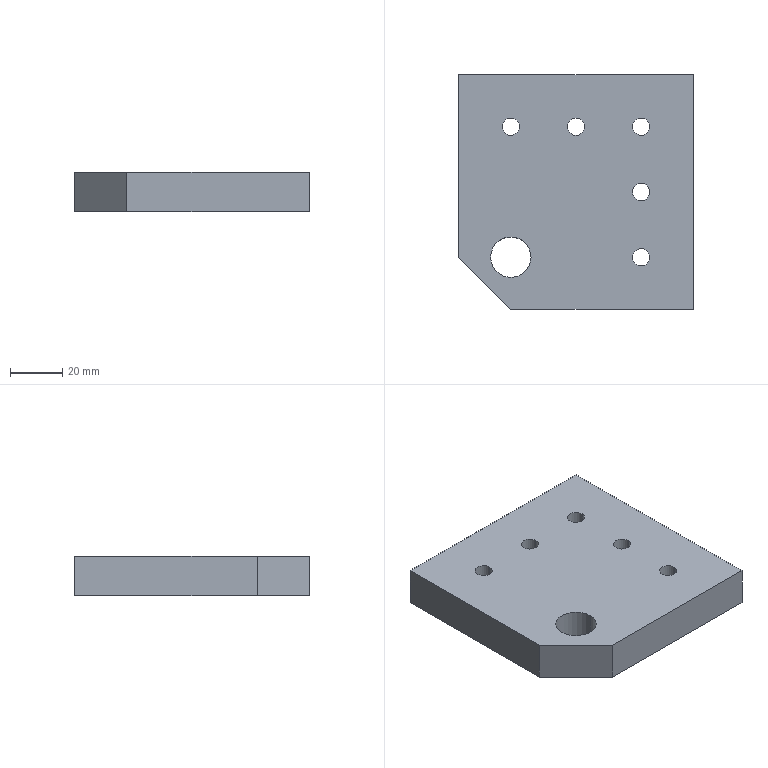Part | SolidWorks | features BaseBody 1 | 1 solid | 34 faces | box 90 x 90 x 15 mm | volume 110422 mm3 | cylinder 22 | plane 12 | commonest cylinder face diameters 6.6 x10 12 x10 15.5 x2
STEP:
#1=CARTESIAN_POINT('',(31.,25.,6.8));
#2=VERTEX_POINT('',#1);
#3=CARTESIAN_POINT('',(19.,25.,6.8));
#4=VERTEX_POINT('',#3);
#5=CARTESIAN_POINT('',(25.,25.,6.8));
#6=DIRECTION('',(0.,0.,-1.));
#7=DIRECTION('',(-1.,0.,0.));
#8=AXIS2_PLACEMENT_3D('',#5,#6,#7);
#9=CIRCLE('',#8,6.);
#10=EDGE_CURVE('',#2,#4,#9,.T.);
#11=ORIENTED_EDGE('',*,*,#10,.F.);
#12=CARTESIAN_POINT('',(31.,25.,0.));
#13=VERTEX_POINT('',#12);
#14=CARTESIAN_POINT('',(31.,25.,0.));
#15=DIRECTION('',(0.,0.,-1.));
#16=VECTOR('',#15,1000.);
#17=LINE('',#14,#16);
#18=EDGE_CURVE('',#2,#13,#17,.T.);
#19=ORIENTED_EDGE('',*,*,#18,.T.);
#20=CARTESIAN_POINT('',(19.,25.,0.));
#21=VERTEX_POINT('',#20);
#22=CARTESIAN_POINT('',(25.,25.,0.));
#23=DIRECTION('',(0.,0.,-1.));
#24=DIRECTION('',(-1.,0.,0.));
#25=AXIS2_PLACEMENT_3D('',#22,#23,#24);
#26=CIRCLE('',#25,6.);
#27=EDGE_CURVE('',#13,#21,#26,.T.);
#28=ORIENTED_EDGE('',*,*,#27,.T.);
#29=CARTESIAN_POINT('',(19.,25.,0.));
#30=DIRECTION('',(0.,0.,-1.));
#31=VECTOR('',#30,1000.);
#32=LINE('',#29,#31);
#33=EDGE_CURVE('',#4,#21,#32,.T.);
#34=ORIENTED_EDGE('',*,*,#33,.F.);
#35=EDGE_LOOP('',(#11,#19,#28,#34));
#36=FACE_OUTER_BOUND('',#35,.T.);
#37=CARTESIAN_POINT('',(25.,25.,0.));
#38=DIRECTION('',(0.,0.,-1.));
#39=DIRECTION('',(-1.,0.,0.));
#40=AXIS2_PLACEMENT_3D('',#37,#38,#39);
#41=CYLINDRICAL_SURFACE('',#40,6.);
#42=ADVANCED_FACE('',(#36),#41,.F.);
#43=CARTESIAN_POINT('',(28.3,25.,15.));
#44=VERTEX_POINT('',#43);
#45=CARTESIAN_POINT('',(21.7,25.,15.));
#46=VERTEX_POINT('',#45);
#47=CARTESIAN_POINT('',(25.,25.,15.));
#48=DIRECTION('',(0.,0.,-1.));
#49=DIRECTION('',(-1.,0.,0.));
#50=AXIS2_PLACEMENT_3D('',#47,#48,#49);
#51=CIRCLE('',#50,3.3);
#52=EDGE_CURVE('',#44,#46,#51,.T.);
#53=ORIENTED_EDGE('',*,*,#52,.F.);
#54=CARTESIAN_POINT('',(28.3,25.,6.8));
#55=VERTEX_POINT('',#54);
#56=CARTESIAN_POINT('',(28.3,25.,0.));
#57=DIRECTION('',(0.,0.,-1.));
#58=VECTOR('',#57,1000.);
#59=LINE('',#56,#58);
#60=EDGE_CURVE('',#44,#55,#59,.T.);
#61=ORIENTED_EDGE('',*,*,#60,.T.);
#62=CARTESIAN_POINT('',(21.7,25.,6.8));
#63=VERTEX_POINT('',#62);
#64=CARTESIAN_POINT('',(25.,25.,6.8));
#65=DIRECTION('',(0.,0.,-1.));
#66=DIRECTION('',(-1.,0.,0.));
#67=AXIS2_PLACEMENT_3D('',#64,#65,#66);
#68=CIRCLE('',#67,3.3);
#69=EDGE_CURVE('',#55,#63,#68,.T.);
#70=ORIENTED_EDGE('',*,*,#69,.T.);
#71=CARTESIAN_POINT('',(21.7,25.,0.));
#72=DIRECTION('',(0.,0.,-1.));
#73=VECTOR('',#72,1000.);
#74=LINE('',#71,#73);
#75=EDGE_CURVE('',#46,#63,#74,.T.);
#76=ORIENTED_EDGE('',*,*,#75,.F.);
#77=EDGE_LOOP('',(#53,#61,#70,#76));
#78=FACE_OUTER_BOUND('',#77,.T.);
#79=CARTESIAN_POINT('',(25.,25.,0.));
#80=DIRECTION('',(0.,0.,-1.));
#81=DIRECTION('',(-1.,0.,0.));
#82=AXIS2_PLACEMENT_3D('',#79,#80,#81);
#83=CYLINDRICAL_SURFACE('',#82,3.3);
#84=ADVANCED_FACE('',(#78),#83,.F.);
#85=CARTESIAN_POINT('',(6.,25.,6.8));
#86=VERTEX_POINT('',#85);
#87=CARTESIAN_POINT('',(-6.,25.,6.8));
#88=VERTEX_POINT('',#87);
#89=CARTESIAN_POINT('',(0.,25.,6.8));
#90=DIRECTION('',(0.,0.,-1.));
#91=DIRECTION('',(-1.,0.,0.));
#92=AXIS2_PLACEMENT_3D('',#89,#90,#91);
#93=CIRCLE('',#92,6.);
#94=EDGE_CURVE('',#86,#88,#93,.T.);
#95=ORIENTED_EDGE('',*,*,#94,.F.);
#96=CARTESIAN_POINT('',(6.,25.,0.));
#97=VERTEX_POINT('',#96);
#98=CARTESIAN_POINT('',(6.,25.,0.));
#99=DIRECTION('',(0.,0.,-1.));
#100=VECTOR('',#99,1000.);
#101=LINE('',#98,#100);
#102=EDGE_CURVE('',#86,#97,#101,.T.);
#103=ORIENTED_EDGE('',*,*,#102,.T.);
#104=CARTESIAN_POINT('',(-6.,25.,0.));
#105=VERTEX_POINT('',#104);
#106=CARTESIAN_POINT('',(0.,25.,0.));
#107=DIRECTION('',(0.,0.,-1.));
#108=DIRECTION('',(-1.,0.,0.));
#109=AXIS2_PLACEMENT_3D('',#106,#107,#108);
#110=CIRCLE('',#109,6.);
#111=EDGE_CURVE('',#97,#105,#110,.T.);
#112=ORIENTED_EDGE('',*,*,#111,.T.);
#113=CARTESIAN_POINT('',(-6.,25.,0.));
#114=DIRECTION('',(0.,0.,-1.));
#115=VECTOR('',#114,1000.);
#116=LINE('',#113,#115);
#117=EDGE_CURVE('',#88,#105,#116,.T.);
#118=ORIENTED_EDGE('',*,*,#117,.F.);
#119=EDGE_LOOP('',(#95,#103,#112,#118));
#120=FACE_OUTER_BOUND('',#119,.T.);
#121=CARTESIAN_POINT('',(0.,25.,0.));
#122=DIRECTION('',(0.,0.,-1.));
#123=DIRECTION('',(-1.,0.,0.));
#124=AXIS2_PLACEMENT_3D('',#121,#122,#123);
#125=CYLINDRICAL_SURFACE('',#124,6.);
#126=ADVANCED_FACE('',(#120),#125,.F.);
#127=CARTESIAN_POINT('',(3.3,25.,15.));
#128=VERTEX_POINT('',#127);
#129=CARTESIAN_POINT('',(-3.3,25.,15.));
#130=VERTEX_POINT('',#129);
#131=CARTESIAN_POINT('',(0.,25.,15.));
#132=DIRECTION('',(0.,0.,-1.));
#133=DIRECTION('',(-1.,0.,0.));
#134=AXIS2_PLACEMENT_3D('',#131,#132,#133);
#135=CIRCLE('',#134,3.3);
#136=EDGE_CURVE('',#128,#130,#135,.T.);
#137=ORIENTED_EDGE('',*,*,#136,.F.);
#138=CARTESIAN_POINT('',(3.3,25.,6.8));
#139=VERTEX_POINT('',#138);
#140=CARTESIAN_POINT('',(3.3,25.,0.));
#141=DIRECTION('',(0.,0.,-1.));
#142=VECTOR('',#141,1000.);
#143=LINE('',#140,#142);
#144=EDGE_CURVE('',#128,#139,#143,.T.);
#145=ORIENTED_EDGE('',*,*,#144,.T.);
#146=CARTESIAN_POINT('',(-3.3,25.,6.8));
#147=VERTEX_POINT('',#146);
#148=CARTESIAN_POINT('',(0.,25.,6.8));
#149=DIRECTION('',(0.,0.,-1.));
#150=DIRECTION('',(-1.,0.,0.));
#151=AXIS2_PLACEMENT_3D('',#148,#149,#150);
#152=CIRCLE('',#151,3.3);
#153=EDGE_CURVE('',#139,#147,#152,.T.);
#154=ORIENTED_EDGE('',*,*,#153,.T.);
#155=CARTESIAN_POINT('',(-3.3,25.,0.));
#156=DIRECTION('',(0.,0.,-1.));
#157=VECTOR('',#156,1000.);
#158=LINE('',#155,#157);
#159=EDGE_CURVE('',#130,#147,#158,.T.);
#160=ORIENTED_EDGE('',*,*,#159,.F.);
#161=EDGE_LOOP('',(#137,#145,#154,#160));
#162=FACE_OUTER_BOUND('',#161,.T.);
#163=CARTESIAN_POINT('',(0.,25.,0.));
#164=DIRECTION('',(0.,0.,-1.));
#165=DIRECTION('',(-1.,0.,0.));
#166=AXIS2_PLACEMENT_3D('',#163,#164,#165);
#167=CYLINDRICAL_SURFACE('',#166,3.3);
#168=ADVANCED_FACE('',(#162),#167,.F.);
#169=CARTESIAN_POINT('',(-19.,25.,6.8));
#170=VERTEX_POINT('',#169);
#171=CARTESIAN_POINT('',(-31.,25.,6.8));
#172=VERTEX_POINT('',#171);
#173=CARTESIAN_POINT('',(-25.,25.,6.8));
#174=DIRECTION('',(0.,0.,-1.));
#175=DIRECTION('',(-1.,0.,0.));
#176=AXIS2_PLACEMENT_3D('',#173,#174,#175);
#177=CIRCLE('',#176,6.);
#178=EDGE_CURVE('',#170,#172,#177,.T.);
#179=ORIENTED_EDGE('',*,*,#178,.F.);
#180=CARTESIAN_POINT('',(-19.,25.,0.));
#181=VERTEX_POINT('',#180);
#182=CARTESIAN_POINT('',(-19.,25.,0.));
#183=DIRECTION('',(0.,0.,-1.));
#184=VECTOR('',#183,1000.);
#185=LINE('',#182,#184);
#186=EDGE_CURVE('',#170,#181,#185,.T.);
#187=ORIENTED_EDGE('',*,*,#186,.T.);
#188=CARTESIAN_POINT('',(-31.,25.,0.));
#189=VERTEX_POINT('',#188);
#190=CARTESIAN_POINT('',(-25.,25.,0.));
#191=DIRECTION('',(0.,0.,-1.));
#192=DIRECTION('',(-1.,0.,0.));
#193=AXIS2_PLACEMENT_3D('',#190,#191,#192);
#194=CIRCLE('',#193,6.);
#195=EDGE_CURVE('',#181,#189,#194,.T.);
#196=ORIENTED_EDGE('',*,*,#195,.T.);
#197=CARTESIAN_POINT('',(-31.,25.,0.));
#198=DIRECTION('',(0.,0.,-1.));
#199=VECTOR('',#198,1000.);
#200=LINE('',#197,#199);
#201=EDGE_CURVE('',#172,#189,#200,.T.);
#202=ORIENTED_EDGE('',*,*,#201,.F.);
#203=EDGE_LOOP('',(#179,#187,#196,#202));
#204=FACE_OUTER_BOUND('',#203,.T.);
#205=CARTESIAN_POINT('',(-25.,25.,0.));
#206=DIRECTION('',(0.,0.,-1.));
#207=DIRECTION('',(-1.,0.,0.));
#208=AXIS2_PLACEMENT_3D('',#205,#206,#207);
#209=CYLINDRICAL_SURFACE('',#208,6.);
#210=ADVANCED_FACE('',(#204),#209,.F.);
#211=CARTESIAN_POINT('',(-21.7,25.,15.));
#212=VERTEX_POINT('',#211);
#213=CARTESIAN_POINT('',(-28.3,25.,15.));
#214=VERTEX_POINT('',#213);
#215=CARTESIAN_POINT('',(-25.,25.,15.));
#216=DIRECTION('',(0.,0.,-1.));
#217=DIRECTION('',(-1.,0.,0.));
#218=AXIS2_PLACEMENT_3D('',#215,#216,#217);
#219=CIRCLE('',#218,3.3);
#220=EDGE_CURVE('',#212,#214,#219,.T.);
#221=ORIENTED_EDGE('',*,*,#220,.F.);
#222=CARTESIAN_POINT('',(-21.7,25.,6.8));
#223=VERTEX_POINT('',#222);
#224=CARTESIAN_POINT('',(-21.7,25.,0.));
#225=DIRECTION('',(0.,0.,-1.));
#226=VECTOR('',#225,1000.);
#227=LINE('',#224,#226);
#228=EDGE_CURVE('',#212,#223,#227,.T.);
#229=ORIENTED_EDGE('',*,*,#228,.T.);
#230=CARTESIAN_POINT('',(-28.3,25.,6.8));
#231=VERTEX_POINT('',#230);
#232=CARTESIAN_POINT('',(-25.,25.,6.8));
#233=DIRECTION('',(0.,0.,-1.));
#234=DIRECTION('',(-1.,0.,0.));
#235=AXIS2_PLACEMENT_3D('',#232,#233,#234);
#236=CIRCLE('',#235,3.3);
#237=EDGE_CURVE('',#223,#231,#236,.T.);
#238=ORIENTED_EDGE('',*,*,#237,.T.);
#239=CARTESIAN_POINT('',(-28.3,25.,0.));
#240=DIRECTION('',(0.,0.,-1.));
#241=VECTOR('',#240,1000.);
#242=LINE('',#239,#241);
#243=EDGE_CURVE('',#214,#231,#242,.T.);
#244=ORIENTED_EDGE('',*,*,#243,.F.);
#245=EDGE_LOOP('',(#221,#229,#238,#244));
#246=FACE_OUTER_BOUND('',#245,.T.);
#247=CARTESIAN_POINT('',(-25.,25.,0.));
#248=DIRECTION('',(0.,0.,-1.));
#249=DIRECTION('',(-1.,0.,0.));
#250=AXIS2_PLACEMENT_3D('',#247,#248,#249);
#251=CYLINDRICAL_SURFACE('',#250,3.3);
#252=ADVANCED_FACE('',(#246),#251,.F.);
#253=CARTESIAN_POINT('',(31.,0.,6.8));
#254=VERTEX_POINT('',#253);
#255=CARTESIAN_POINT('',(19.,0.,6.8));
#256=VERTEX_POINT('',#255);
#257=CARTESIAN_POINT('',(25.,0.,6.8));
#258=DIRECTION('',(0.,0.,-1.));
#259=DIRECTION('',(-1.,0.,0.));
#260=AXIS2_PLACEMENT_3D('',#257,#258,#259);
#261=CIRCLE('',#260,6.);
#262=EDGE_CURVE('',#254,#256,#261,.T.);
#263=ORIENTED_EDGE('',*,*,#262,.F.);
#264=CARTESIAN_POINT('',(31.,0.,0.));
#265=VERTEX_POINT('',#264);
#266=CARTESIAN_POINT('',(31.,0.,0.));
#267=DIRECTION('',(0.,0.,-1.));
#268=VECTOR('',#267,1000.);
#269=LINE('',#266,#268);
#270=EDGE_CURVE('',#254,#265,#269,.T.);
#271=ORIENTED_EDGE('',*,*,#270,.T.);
#272=CARTESIAN_POINT('',(19.,0.,0.));
#273=VERTEX_POINT('',#272);
#274=CARTESIAN_POINT('',(25.,0.,0.));
#275=DIRECTION('',(0.,0.,-1.));
#276=DIRECTION('',(-1.,0.,0.));
#277=AXIS2_PLACEMENT_3D('',#274,#275,#276);
#278=CIRCLE('',#277,6.);
#279=EDGE_CURVE('',#265,#273,#278,.T.);
#280=ORIENTED_EDGE('',*,*,#279,.T.);
#281=CARTESIAN_POINT('',(19.,0.,0.));
#282=DIRECTION('',(0.,0.,-1.));
#283=VECTOR('',#282,1000.);
#284=LINE('',#281,#283);
#285=EDGE_CURVE('',#256,#273,#284,.T.);
#286=ORIENTED_EDGE('',*,*,#285,.F.);
#287=EDGE_LOOP('',(#263,#271,#280,#286));
#288=FACE_OUTER_BOUND('',#287,.T.);
#289=CARTESIAN_POINT('',(25.,0.,0.));
#290=DIRECTION('',(0.,0.,-1.));
#291=DIRECTION('',(-1.,0.,0.));
#292=AXIS2_PLACEMENT_3D('',#289,#290,#291);
#293=CYLINDRICAL_SURFACE('',#292,6.);
#294=ADVANCED_FACE('',(#288),#293,.F.);
#295=CARTESIAN_POINT('',(28.3,0.,15.));
#296=VERTEX_POINT('',#295);
#297=CARTESIAN_POINT('',(21.7,0.,15.));
#298=VERTEX_POINT('',#297);
#299=CARTESIAN_POINT('',(25.,0.,15.));
#300=DIRECTION('',(0.,0.,-1.));
#301=DIRECTION('',(-1.,0.,0.));
#302=AXIS2_PLACEMENT_3D('',#299,#300,#301);
#303=CIRCLE('',#302,3.3);
#304=EDGE_CURVE('',#296,#298,#303,.T.);
#305=ORIENTED_EDGE('',*,*,#304,.F.);
#306=CARTESIAN_POINT('',(28.3,0.,6.8));
#307=VERTEX_POINT('',#306);
#308=CARTESIAN_POINT('',(28.3,0.,0.));
#309=DIRECTION('',(0.,0.,-1.));
#310=VECTOR('',#309,1000.);
#311=LINE('',#308,#310);
#312=EDGE_CURVE('',#296,#307,#311,.T.);
#313=ORIENTED_EDGE('',*,*,#312,.T.);
#314=CARTESIAN_POINT('',(21.7,0.,6.8));
#315=VERTEX_POINT('',#314);
#316=CARTESIAN_POINT('',(25.,0.,6.8));
#317=DIRECTION('',(0.,0.,-1.));
#318=DIRECTION('',(-1.,0.,0.));
#319=AXIS2_PLACEMENT_3D('',#316,#317,#318);
#320=CIRCLE('',#319,3.3);
#321=EDGE_CURVE('',#307,#315,#320,.T.);
#322=ORIENTED_EDGE('',*,*,#321,.T.);
#323=CARTESIAN_POINT('',(21.7,0.,0.));
#324=DIRECTION('',(0.,0.,-1.));
#325=VECTOR('',#324,1000.);
#326=LINE('',#323,#325);
#327=EDGE_CURVE('',#298,#315,#326,.T.);
#328=ORIENTED_EDGE('',*,*,#327,.F.);
#329=EDGE_LOOP('',(#305,#313,#322,#328));
#330=FACE_OUTER_BOUND('',#329,.T.);
#331=CARTESIAN_POINT('',(25.,0.,0.));
#332=DIRECTION('',(0.,0.,-1.));
#333=DIRECTION('',(-1.,0.,0.));
#334=AXIS2_PLACEMENT_3D('',#331,#332,#333);
#335=CYLINDRICAL_SURFACE('',#334,3.3);
#336=ADVANCED_FACE('',(#330),#335,.F.);
#337=CARTESIAN_POINT('',(31.,-25.,6.8));
#338=VERTEX_POINT('',#337);
#339=CARTESIAN_POINT('',(19.,-25.,6.8));
#340=VERTEX_POINT('',#339);
#341=CARTESIAN_POINT('',(25.,-25.,6.8));
#342=DIRECTION('',(0.,0.,-1.));
#343=DIRECTION('',(-1.,0.,0.));
#344=AXIS2_PLACEMENT_3D('',#341,#342,#343);
#345=CIRCLE('',#344,6.);
#346=EDGE_CURVE('',#338,#340,#345,.T.);
#347=ORIENTED_EDGE('',*,*,#346,.F.);
#348=CARTESIAN_POINT('',(31.,-25.,0.));
#349=VERTEX_POINT('',#348);
#350=CARTESIAN_POINT('',(31.,-25.,0.));
#351=DIRECTION('',(0.,0.,-1.));
#352=VECTOR('',#351,1000.);
#353=LINE('',#350,#352);
#354=EDGE_CURVE('',#338,#349,#353,.T.);
#355=ORIENTED_EDGE('',*,*,#354,.T.);
#356=CARTESIAN_POINT('',(19.,-25.,0.));
#357=VERTEX_POINT('',#356);
#358=CARTESIAN_POINT('',(25.,-25.,0.));
#359=DIRECTION('',(0.,0.,-1.));
#360=DIRECTION('',(-1.,0.,0.));
#361=AXIS2_PLACEMENT_3D('',#358,#359,#360);
#362=CIRCLE('',#361,6.);
#363=EDGE_CURVE('',#349,#357,#362,.T.);
#364=ORIENTED_EDGE('',*,*,#363,.T.);
#365=CARTESIAN_POINT('',(19.,-25.,0.));
#366=DIRECTION('',(0.,0.,-1.));
#367=VECTOR('',#366,1000.);
#368=LINE('',#365,#367);
#369=EDGE_CURVE('',#340,#357,#368,.T.);
#370=ORIENTED_EDGE('',*,*,#369,.F.);
#371=EDGE_LOOP('',(#347,#355,#364,#370));
#372=FACE_OUTER_BOUND('',#371,.T.);
#373=CARTESIAN_POINT('',(25.,-25.,0.));
#374=DIRECTION('',(0.,0.,-1.));
#375=DIRECTION('',(-1.,0.,0.));
#376=AXIS2_PLACEMENT_3D('',#373,#374,#375);
#377=CYLINDRICAL_SURFACE('',#376,6.);
#378=ADVANCED_FACE('',(#372),#377,.F.);
#379=CARTESIAN_POINT('',(28.3,-25.,15.));
#380=VERTEX_POINT('',#379);
#381=CARTESIAN_POINT('',(21.7,-25.,15.));
#382=VERTEX_POINT('',#381);
#383=CARTESIAN_POINT('',(25.,-25.,15.));
#384=DIRECTION('',(0.,0.,-1.));
#385=DIRECTION('',(-1.,0.,0.));
#386=AXIS2_PLACEMENT_3D('',#383,#384,#385);
#387=CIRCLE('',#386,3.3);
#388=EDGE_CURVE('',#380,#382,#387,.T.);
#389=ORIENTED_EDGE('',*,*,#388,.F.);
#390=CARTESIAN_POINT('',(28.3,-25.,6.8));
#391=VERTEX_POINT('',#390);
#392=CARTESIAN_POINT('',(28.3,-25.,0.));
#393=DIRECTION('',(0.,0.,-1.));
#394=VECTOR('',#393,1000.);
#395=LINE('',#392,#394);
#396=EDGE_CURVE('',#380,#391,#395,.T.);
#397=ORIENTED_EDGE('',*,*,#396,.T.);
#398=CARTESIAN_POINT('',(21.7,-25.,6.8));
#399=VERTEX_POINT('',#398);
#400=CARTESIAN_POINT('',(25.,-25.,6.8));
#401=DIRECTION('',(0.,0.,-1.));
#402=DIRECTION('',(-1.,0.,0.));
#403=AXIS2_PLACEMENT_3D('',#400,#401,#402);
#404=CIRCLE('',#403,3.3);
#405=EDGE_CURVE('',#391,#399,#404,.T.);
#406=ORIENTED_EDGE('',*,*,#405,.T.);
#407=CARTESIAN_POINT('',(21.7,-25.,0.));
#408=DIRECTION('',(0.,0.,-1.));
#409=VECTOR('',#408,1000.);
#410=LINE('',#407,#409);
#411=EDGE_CURVE('',#382,#399,#410,.T.);
#412=ORIENTED_EDGE('',*,*,#411,.F.);
#413=EDGE_LOOP('',(#389,#397,#406,#412));
#414=FACE_OUTER_BOUND('',#413,.T.);
#415=CARTESIAN_POINT('',(25.,-25.,0.));
#416=DIRECTION('',(0.,0.,-1.));
#417=DIRECTION('',(-1.,0.,0.));
#418=AXIS2_PLACEMENT_3D('',#415,#416,#417);
#419=CYLINDRICAL_SURFACE('',#418,3.3);
#420=ADVANCED_FACE('',(#414),#419,.F.);
#421=CARTESIAN_POINT('',(-32.75,-25.,15.));
#422=VERTEX_POINT('',#421);
#423=CARTESIAN_POINT('',(-17.25,-25.,15.));
#424=VERTEX_POINT('',#423);
#425=CARTESIAN_POINT('',(-25.,-25.,15.));
#426=DIRECTION('',(0.,0.,1.));
#427=DIRECTION('',(1.,0.,0.));
#428=AXIS2_PLACEMENT_3D('',#425,#426,#427);
#429=CIRCLE('',#428,7.75);
#430=EDGE_CURVE('',#422,#424,#429,.T.);
#431=ORIENTED_EDGE('',*,*,#430,.T.);
#432=CARTESIAN_POINT('',(-17.25,-25.,0.));
#433=VERTEX_POINT('',#432);
#434=CARTESIAN_POINT('',(-17.25,-25.,0.));
#435=DIRECTION('',(0.,0.,-1.));
#436=VECTOR('',#435,1000.);
#437=LINE('',#434,#436);
#438=EDGE_CURVE('',#424,#433,#437,.T.);
#439=ORIENTED_EDGE('',*,*,#438,.T.);
#440=CARTESIAN_POINT('',(-32.75,-25.,0.));
#441=VERTEX_POINT('',#440);
#442=CARTESIAN_POINT('',(-25.,-25.,0.));
#443=DIRECTION('',(0.,0.,-1.));
#444=DIRECTION('',(-1.,0.,0.));
#445=AXIS2_PLACEMENT_3D('',#442,#443,#444);
#446=CIRCLE('',#445,7.75);
#447=EDGE_CURVE('',#433,#441,#446,.T.);
#448=ORIENTED_EDGE('',*,*,#447,.T.);
#449=CARTESIAN_POINT('',(-32.75,-25.,0.));
#450=DIRECTION('',(0.,0.,-1.));
#451=VECTOR('',#450,1000.);
#452=LINE('',#449,#451);
#453=EDGE_CURVE('',#422,#441,#452,.T.);
#454=ORIENTED_EDGE('',*,*,#453,.F.);
#455=EDGE_LOOP('',(#431,#439,#448,#454));
#456=FACE_OUTER_BOUND('',#455,.T.);
#457=CARTESIAN_POINT('',(-25.,-25.,0.));
#458=DIRECTION('',(0.,0.,-1.));
#459=DIRECTION('',(-1.,0.,0.));
#460=AXIS2_PLACEMENT_3D('',#457,#458,#459);
#461=CYLINDRICAL_SURFACE('',#460,7.75);
#462=ADVANCED_FACE('',(#456),#461,.F.);
#463=CARTESIAN_POINT('',(25.,25.,6.8));
#464=DIRECTION('',(0.,0.,-1.));
#465=DIRECTION('',(-1.,0.,0.));
#466=AXIS2_PLACEMENT_3D('',#463,#464,#465);
#467=CIRCLE('',#466,3.3);
#468=EDGE_CURVE('',#63,#55,#467,.T.);
#469=ORIENTED_EDGE('',*,*,#468,.F.);
#470=ORIENTED_EDGE('',*,*,#69,.F.);
#471=EDGE_LOOP('',(#469,#470));
#472=FACE_BOUND('',#471,.T.);
#473=CARTESIAN_POINT('',(25.,25.,6.8));
#474=DIRECTION('',(0.,0.,-1.));
#475=DIRECTION('',(-1.,0.,0.));
#476=AXIS2_PLACEMENT_3D('',#473,#474,#475);
#477=CIRCLE('',#476,6.);
#478=EDGE_CURVE('',#4,#2,#477,.T.);
#479=ORIENTED_EDGE('',*,*,#478,.T.);
#480=ORIENTED_EDGE('',*,*,#10,.T.);
#481=EDGE_LOOP('',(#479,#480));
#482=FACE_OUTER_BOUND('',#481,.T.);
#483=CARTESIAN_POINT('',(28.3,25.,6.8));
#484=DIRECTION('',(0.,0.,1.));
#485=DIRECTION('',(1.,0.,0.));
#486=AXIS2_PLACEMENT_3D('',#483,#484,#485);
#487=PLANE('',#486);
#488=ADVANCED_FACE('',(#472,#482),#487,.F.);
#489=CARTESIAN_POINT('',(0.,25.,6.8));
#490=DIRECTION('',(0.,0.,-1.));
#491=DIRECTION('',(-1.,0.,0.));
#492=AXIS2_PLACEMENT_3D('',#489,#490,#491);
#493=CIRCLE('',#492,3.3);
#494=EDGE_CURVE('',#147,#139,#493,.T.);
#495=ORIENTED_EDGE('',*,*,#494,.F.);
#496=ORIENTED_EDGE('',*,*,#153,.F.);
#497=EDGE_LOOP('',(#495,#496));
#498=FACE_BOUND('',#497,.T.);
#499=CARTESIAN_POINT('',(0.,25.,6.8));
#500=DIRECTION('',(0.,0.,-1.));
#501=DIRECTION('',(-1.,0.,0.));
#502=AXIS2_PLACEMENT_3D('',#499,#500,#501);
#503=CIRCLE('',#502,6.);
#504=EDGE_CURVE('',#88,#86,#503,.T.);
#505=ORIENTED_EDGE('',*,*,#504,.T.);
#506=ORIENTED_EDGE('',*,*,#94,.T.);
#507=EDGE_LOOP('',(#505,#506));
#508=FACE_OUTER_BOUND('',#507,.T.);
#509=CARTESIAN_POINT('',(3.3,25.,6.8));
#510=DIRECTION('',(0.,0.,1.));
#511=DIRECTION('',(1.,0.,0.));
#512=AXIS2_PLACEMENT_3D('',#509,#510,#511);
#513=PLANE('',#512);
#514=ADVANCED_FACE('',(#498,#508),#513,.F.);
#515=CARTESIAN_POINT('',(-25.,25.,6.8));
#516=DIRECTION('',(0.,0.,-1.));
#517=DIRECTION('',(-1.,0.,0.));
#518=AXIS2_PLACEMENT_3D('',#515,#516,#517);
#519=CIRCLE('',#518,3.3);
#520=EDGE_CURVE('',#231,#223,#519,.T.);
#521=ORIENTED_EDGE('',*,*,#520,.F.);
#522=ORIENTED_EDGE('',*,*,#237,.F.);
#523=EDGE_LOOP('',(#521,#522));
#524=FACE_BOUND('',#523,.T.);
#525=CARTESIAN_POINT('',(-25.,25.,6.8));
#526=DIRECTION('',(0.,0.,-1.));
#527=DIRECTION('',(-1.,0.,0.));
#528=AXIS2_PLACEMENT_3D('',#525,#526,#527);
#529=CIRCLE('',#528,6.);
#530=EDGE_CURVE('',#172,#170,#529,.T.);
#531=ORIENTED_EDGE('',*,*,#530,.T.);
#532=ORIENTED_EDGE('',*,*,#178,.T.);
#533=EDGE_LOOP('',(#531,#532));
#534=FACE_OUTER_BOUND('',#533,.T.);
#535=CARTESIAN_POINT('',(-21.7,25.,6.8));
#536=DIRECTION('',(0.,0.,1.));
#537=DIRECTION('',(1.,0.,0.));
#538=AXIS2_PLACEMENT_3D('',#535,#536,#537);
#539=PLANE('',#538);
#540=ADVANCED_FACE('',(#524,#534),#539,.F.);
#541=CARTESIAN_POINT('',(25.,0.,6.8));
#542=DIRECTION('',(0.,0.,-1.));
#543=DIRECTION('',(-1.,0.,0.));
#544=AXIS2_PLACEMENT_3D('',#541,#542,#543);
#545=CIRCLE('',#544,3.3);
#546=EDGE_CURVE('',#315,#307,#545,.T.);
#547=ORIENTED_EDGE('',*,*,#546,.F.);
#548=ORIENTED_EDGE('',*,*,#321,.F.);
#549=EDGE_LOOP('',(#547,#548));
#550=FACE_BOUND('',#549,.T.);
#551=CARTESIAN_POINT('',(25.,0.,6.8));
#552=DIRECTION('',(0.,0.,-1.));
#553=DIRECTION('',(-1.,0.,0.));
#554=AXIS2_PLACEMENT_3D('',#551,#552,#553);
#555=CIRCLE('',#554,6.);
#556=EDGE_CURVE('',#256,#254,#555,.T.);
#557=ORIENTED_EDGE('',*,*,#556,.T.);
#558=ORIENTED_EDGE('',*,*,#262,.T.);
#559=EDGE_LOOP('',(#557,#558));
#560=FACE_OUTER_BOUND('',#559,.T.);
#561=CARTESIAN_POINT('',(28.3,0.,6.8));
#562=DIRECTION('',(0.,0.,1.));
#563=DIRECTION('',(1.,0.,0.));
#564=AXIS2_PLACEMENT_3D('',#561,#562,#563);
#565=PLANE('',#564);
#566=ADVANCED_FACE('',(#550,#560),#565,.F.);
#567=CARTESIAN_POINT('',(25.,-25.,6.8));
#568=DIRECTION('',(0.,0.,-1.));
#569=DIRECTION('',(-1.,0.,0.));
#570=AXIS2_PLACEMENT_3D('',#567,#568,#569);
#571=CIRCLE('',#570,3.3);
#572=EDGE_CURVE('',#399,#391,#571,.T.);
#573=ORIENTED_EDGE('',*,*,#572,.F.);
#574=ORIENTED_EDGE('',*,*,#405,.F.);
#575=EDGE_LOOP('',(#573,#574));
#576=FACE_BOUND('',#575,.T.);
#577=CARTESIAN_POINT('',(25.,-25.,6.8));
#578=DIRECTION('',(0.,0.,-1.));
#579=DIRECTION('',(-1.,0.,0.));
#580=AXIS2_PLACEMENT_3D('',#577,#578,#579);
#581=CIRCLE('',#580,6.);
#582=EDGE_CURVE('',#340,#338,#581,.T.);
#583=ORIENTED_EDGE('',*,*,#582,.T.);
#584=ORIENTED_EDGE('',*,*,#346,.T.);
#585=EDGE_LOOP('',(#583,#584));
#586=FACE_OUTER_BOUND('',#585,.T.);
#587=CARTESIAN_POINT('',(28.3,-25.,6.8));
#588=DIRECTION('',(0.,0.,1.));
#589=DIRECTION('',(1.,0.,0.));
#590=AXIS2_PLACEMENT_3D('',#587,#588,#589);
#591=PLANE('',#590);
#592=ADVANCED_FACE('',(#576,#586),#591,.F.);
#593=CARTESIAN_POINT('',(-45.,-25.,15.));
#594=VERTEX_POINT('',#593);
#595=CARTESIAN_POINT('',(-25.,-45.,15.));
#596=VERTEX_POINT('',#595);
#597=CARTESIAN_POINT('',(-35.,-35.,15.));
#598=DIRECTION('',(0.7071,-0.7071,0.));
#599=VECTOR('',#598,1000.);
#600=LINE('',#597,#599);
#601=EDGE_CURVE('',#594,#596,#600,.T.);
#602=ORIENTED_EDGE('',*,*,#601,.F.);
#603=CARTESIAN_POINT('',(-45.,-25.,0.));
#604=VERTEX_POINT('',#603);
#605=CARTESIAN_POINT('',(-45.,-25.,15.));
#606=DIRECTION('',(0.,0.,1.));
#607=VECTOR('',#606,1000.);
#608=LINE('',#605,#607);
#609=EDGE_CURVE('',#604,#594,#608,.T.);
#610=ORIENTED_EDGE('',*,*,#609,.F.);
#611=CARTESIAN_POINT('',(-25.,-45.,0.));
#612=VERTEX_POINT('',#611);
#613=CARTESIAN_POINT('',(-25.,-45.,0.));
#614=DIRECTION('',(-0.7071,0.7071,0.));
#615=VECTOR('',#614,1000.);
#616=LINE('',#613,#615);
#617=EDGE_CURVE('',#612,#604,#616,.T.);
#618=ORIENTED_EDGE('',*,*,#617,.F.);
#619=CARTESIAN_POINT('',(-25.,-45.,15.));
#620=DIRECTION('',(0.,0.,-1.));
#621=VECTOR('',#620,1000.);
#622=LINE('',#619,#621);
#623=EDGE_CURVE('',#596,#612,#622,.T.);
#624=ORIENTED_EDGE('',*,*,#623,.F.);
#625=EDGE_LOOP('',(#602,#610,#618,#624));
#626=FACE_OUTER_BOUND('',#625,.T.);
#627=CARTESIAN_POINT('',(-25.,-45.,15.));
#628=DIRECTION('',(0.7071,0.7071,0.));
#629=DIRECTION('',(0.,0.,-1.));
#630=AXIS2_PLACEMENT_3D('',#627,#628,#629);
#631=PLANE('',#630);
#632=ADVANCED_FACE('',(#626),#631,.F.);
#633=CARTESIAN_POINT('',(-25.,-25.,0.));
#634=DIRECTION('',(0.,0.,-1.));
#635=DIRECTION('',(-1.,0.,0.));
#636=AXIS2_PLACEMENT_3D('',#633,#634,#635);
#637=CIRCLE('',#636,7.75);
#638=EDGE_CURVE('',#441,#433,#637,.T.);
#639=ORIENTED_EDGE('',*,*,#638,.F.);
#640=ORIENTED_EDGE('',*,*,#447,.F.);
#641=EDGE_LOOP('',(#639,#640));
#642=FACE_BOUND('',#641,.T.);
#643=CARTESIAN_POINT('',(25.,-25.,0.));
#644=DIRECTION('',(0.,0.,-1.));
#645=DIRECTION('',(-1.,0.,0.));
#646=AXIS2_PLACEMENT_3D('',#643,#644,#645);
#647=CIRCLE('',#646,6.);
#648=EDGE_CURVE('',#357,#349,#647,.T.);
#649=ORIENTED_EDGE('',*,*,#648,.F.);
#650=ORIENTED_EDGE('',*,*,#363,.F.);
#651=EDGE_LOOP('',(#649,#650));
#652=FACE_BOUND('',#651,.T.);
#653=CARTESIAN_POINT('',(25.,0.,0.));
#654=DIRECTION('',(0.,0.,-1.));
#655=DIRECTION('',(-1.,0.,0.));
#656=AXIS2_PLACEMENT_3D('',#653,#654,#655);
#657=CIRCLE('',#656,6.);
#658=EDGE_CURVE('',#273,#265,#657,.T.);
#659=ORIENTED_EDGE('',*,*,#658,.F.);
#660=ORIENTED_EDGE('',*,*,#279,.F.);
#661=EDGE_LOOP('',(#659,#660));
#662=FACE_BOUND('',#661,.T.);
#663=CARTESIAN_POINT('',(-25.,25.,0.));
#664=DIRECTION('',(0.,0.,-1.));
#665=DIRECTION('',(-1.,0.,0.));
#666=AXIS2_PLACEMENT_3D('',#663,#664,#665);
#667=CIRCLE('',#666,6.);
#668=EDGE_CURVE('',#189,#181,#667,.T.);
#669=ORIENTED_EDGE('',*,*,#668,.F.);
#670=ORIENTED_EDGE('',*,*,#195,.F.);
#671=EDGE_LOOP('',(#669,#670));
#672=FACE_BOUND('',#671,.T.);
#673=CARTESIAN_POINT('',(0.,25.,0.));
#674=DIRECTION('',(0.,0.,-1.));
#675=DIRECTION('',(-1.,0.,0.));
#676=AXIS2_PLACEMENT_3D('',#673,#674,#675);
#677=CIRCLE('',#676,6.);
#678=EDGE_CURVE('',#105,#97,#677,.T.);
#679=ORIENTED_EDGE('',*,*,#678,.F.);
#680=ORIENTED_EDGE('',*,*,#111,.F.);
#681=EDGE_LOOP('',(#679,#680));
#682=FACE_BOUND('',#681,.T.);
#683=CARTESIAN_POINT('',(25.,25.,0.));
#684=DIRECTION('',(0.,0.,-1.));
#685=DIRECTION('',(-1.,0.,0.));
#686=AXIS2_PLACEMENT_3D('',#683,#684,#685);
#687=CIRCLE('',#686,6.);
#688=EDGE_CURVE('',#21,#13,#687,.T.);
#689=ORIENTED_EDGE('',*,*,#688,.F.);
#690=ORIENTED_EDGE('',*,*,#27,.F.);
#691=EDGE_LOOP('',(#689,#690));
#692=FACE_BOUND('',#691,.T.);
#693=CARTESIAN_POINT('',(45.,-45.,0.));
#694=VERTEX_POINT('',#693);
#695=CARTESIAN_POINT('',(-45.,-45.,0.));
#696=DIRECTION('',(1.,0.,0.));
#697=VECTOR('',#696,1000.);
#698=LINE('',#695,#697);
#699=EDGE_CURVE('',#612,#694,#698,.T.);
#700=ORIENTED_EDGE('',*,*,#699,.F.);
#701=ORIENTED_EDGE('',*,*,#617,.T.);
#702=CARTESIAN_POINT('',(-45.,45.,0.));
#703=VERTEX_POINT('',#702);
#704=CARTESIAN_POINT('',(-45.,45.,0.));
#705=DIRECTION('',(0.,-1.,0.));
#706=VECTOR('',#705,1000.);
#707=LINE('',#704,#706);
#708=EDGE_CURVE('',#703,#604,#707,.T.);
#709=ORIENTED_EDGE('',*,*,#708,.F.);
#710=CARTESIAN_POINT('',(45.,45.,0.));
#711=VERTEX_POINT('',#710);
#712=CARTESIAN_POINT('',(-45.,45.,0.));
#713=DIRECTION('',(-1.,0.,0.));
#714=VECTOR('',#713,1000.);
#715=LINE('',#712,#714);
#716=EDGE_CURVE('',#711,#703,#715,.T.);
#717=ORIENTED_EDGE('',*,*,#716,.F.);
#718=CARTESIAN_POINT('',(45.,45.,0.));
#719=DIRECTION('',(0.,1.,0.));
#720=VECTOR('',#719,1000.);
#721=LINE('',#718,#720);
#722=EDGE_CURVE('',#694,#711,#721,.T.);
#723=ORIENTED_EDGE('',*,*,#722,.F.);
#724=EDGE_LOOP('',(#700,#701,#709,#717,#723));
#725=FACE_OUTER_BOUND('',#724,.T.);
#726=CARTESIAN_POINT('',(0.,0.,0.));
#727=DIRECTION('',(0.,0.,1.));
#728=DIRECTION('',(1.,0.,0.));
#729=AXIS2_PLACEMENT_3D('',#726,#727,#728);
#730=PLANE('',#729);
#731=ADVANCED_FACE('',(#642,#652,#662,#672,#682,#692,#725),#730,.F.);
#732=ORIENTED_EDGE('',*,*,#430,.F.);
#733=CARTESIAN_POINT('',(-25.,-25.,15.));
#734=DIRECTION('',(0.,0.,1.));
#735=DIRECTION('',(1.,0.,0.));
#736=AXIS2_PLACEMENT_3D('',#733,#734,#735);
#737=CIRCLE('',#736,7.75);
#738=EDGE_CURVE('',#424,#422,#737,.T.);
#739=ORIENTED_EDGE('',*,*,#738,.F.);
#740=EDGE_LOOP('',(#732,#739));
#741=FACE_BOUND('',#740,.T.);
#742=CARTESIAN_POINT('',(25.,-25.,15.));
#743=DIRECTION('',(0.,0.,-1.));
#744=DIRECTION('',(-1.,0.,0.));
#745=AXIS2_PLACEMENT_3D('',#742,#743,#744);
#746=CIRCLE('',#745,3.3);
#747=EDGE_CURVE('',#382,#380,#746,.T.);
#748=ORIENTED_EDGE('',*,*,#747,.T.);
#749=ORIENTED_EDGE('',*,*,#388,.T.);
#750=EDGE_LOOP('',(#748,#749));
#751=FACE_BOUND('',#750,.T.);
#752=CARTESIAN_POINT('',(25.,0.,15.));
#753=DIRECTION('',(0.,0.,-1.));
#754=DIRECTION('',(-1.,0.,0.));
#755=AXIS2_PLACEMENT_3D('',#752,#753,#754);
#756=CIRCLE('',#755,3.3);
#757=EDGE_CURVE('',#298,#296,#756,.T.);
#758=ORIENTED_EDGE('',*,*,#757,.T.);
#759=ORIENTED_EDGE('',*,*,#304,.T.);
#760=EDGE_LOOP('',(#758,#759));
#761=FACE_BOUND('',#760,.T.);
#762=CARTESIAN_POINT('',(-25.,25.,15.));
#763=DIRECTION('',(0.,0.,-1.));
#764=DIRECTION('',(-1.,0.,0.));
#765=AXIS2_PLACEMENT_3D('',#762,#763,#764);
#766=CIRCLE('',#765,3.3);
#767=EDGE_CURVE('',#214,#212,#766,.T.);
#768=ORIENTED_EDGE('',*,*,#767,.T.);
#769=ORIENTED_EDGE('',*,*,#220,.T.);
#770=EDGE_LOOP('',(#768,#769));
#771=FACE_BOUND('',#770,.T.);
#772=CARTESIAN_POINT('',(0.,25.,15.));
#773=DIRECTION('',(0.,0.,-1.));
#774=DIRECTION('',(-1.,0.,0.));
#775=AXIS2_PLACEMENT_3D('',#772,#773,#774);
#776=CIRCLE('',#775,3.3);
#777=EDGE_CURVE('',#130,#128,#776,.T.);
#778=ORIENTED_EDGE('',*,*,#777,.T.);
#779=ORIENTED_EDGE('',*,*,#136,.T.);
#780=EDGE_LOOP('',(#778,#779));
#781=FACE_BOUND('',#780,.T.);
#782=CARTESIAN_POINT('',(25.,25.,15.));
#783=DIRECTION('',(0.,0.,-1.));
#784=DIRECTION('',(-1.,0.,0.));
#785=AXIS2_PLACEMENT_3D('',#782,#783,#784);
#786=CIRCLE('',#785,3.3);
#787=EDGE_CURVE('',#46,#44,#786,.T.);
#788=ORIENTED_EDGE('',*,*,#787,.T.);
#789=ORIENTED_EDGE('',*,*,#52,.T.);
#790=EDGE_LOOP('',(#788,#789));
#791=FACE_BOUND('',#790,.T.);
#792=CARTESIAN_POINT('',(-45.,45.,15.));
#793=VERTEX_POINT('',#792);
#794=CARTESIAN_POINT('',(-45.,45.,15.));
#795=DIRECTION('',(0.,-1.,0.));
#796=VECTOR('',#795,1000.);
#797=LINE('',#794,#796);
#798=EDGE_CURVE('',#793,#594,#797,.T.);
#799=ORIENTED_EDGE('',*,*,#798,.T.);
#800=ORIENTED_EDGE('',*,*,#601,.T.);
#801=CARTESIAN_POINT('',(45.,-45.,15.));
#802=VERTEX_POINT('',#801);
#803=CARTESIAN_POINT('',(-45.,-45.,15.));
#804=DIRECTION('',(1.,0.,0.));
#805=VECTOR('',#804,1000.);
#806=LINE('',#803,#805);
#807=EDGE_CURVE('',#596,#802,#806,.T.);
#808=ORIENTED_EDGE('',*,*,#807,.T.);
#809=CARTESIAN_POINT('',(45.,45.,15.));
#810=VERTEX_POINT('',#809);
#811=CARTESIAN_POINT('',(45.,45.,15.));
#812=DIRECTION('',(0.,1.,0.));
#813=VECTOR('',#812,1000.);
#814=LINE('',#811,#813);
#815=EDGE_CURVE('',#802,#810,#814,.T.);
#816=ORIENTED_EDGE('',*,*,#815,.T.);
#817=CARTESIAN_POINT('',(-45.,45.,15.));
#818=DIRECTION('',(-1.,0.,0.));
#819=VECTOR('',#818,1000.);
#820=LINE('',#817,#819);
#821=EDGE_CURVE('',#810,#793,#820,.T.);
#822=ORIENTED_EDGE('',*,*,#821,.T.);
#823=EDGE_LOOP('',(#799,#800,#808,#816,#822));
#824=FACE_OUTER_BOUND('',#823,.T.);
#825=CARTESIAN_POINT('',(0.,0.,15.));
#826=DIRECTION('',(0.,0.,1.));
#827=DIRECTION('',(1.,0.,0.));
#828=AXIS2_PLACEMENT_3D('',#825,#826,#827);
#829=PLANE('',#828);
#830=ADVANCED_FACE('',(#741,#751,#761,#771,#781,#791,#824),#829,.T.);
#831=ORIENTED_EDGE('',*,*,#807,.F.);
#832=ORIENTED_EDGE('',*,*,#623,.T.);
#833=ORIENTED_EDGE('',*,*,#699,.T.);
#834=CARTESIAN_POINT('',(45.,-45.,15.));
#835=DIRECTION('',(0.,0.,-1.));
#836=VECTOR('',#835,1000.);
#837=LINE('',#834,#836);
#838=EDGE_CURVE('',#802,#694,#837,.T.);
#839=ORIENTED_EDGE('',*,*,#838,.F.);
#840=EDGE_LOOP('',(#831,#832,#833,#839));
#841=FACE_OUTER_BOUND('',#840,.T.);
#842=CARTESIAN_POINT('',(-45.,-45.,15.));
#843=DIRECTION('',(0.,1.,0.));
#844=DIRECTION('',(1.,0.,0.));
#845=AXIS2_PLACEMENT_3D('',#842,#843,#844);
#846=PLANE('',#845);
#847=ADVANCED_FACE('',(#841),#846,.F.);
#848=ORIENTED_EDGE('',*,*,#708,.T.);
#849=ORIENTED_EDGE('',*,*,#609,.T.);
#850=ORIENTED_EDGE('',*,*,#798,.F.);
#851=CARTESIAN_POINT('',(-45.,45.,15.));
#852=DIRECTION('',(0.,0.,-1.));
#853=VECTOR('',#852,1000.);
#854=LINE('',#851,#853);
#855=EDGE_CURVE('',#793,#703,#854,.T.);
#856=ORIENTED_EDGE('',*,*,#855,.T.);
#857=EDGE_LOOP('',(#848,#849,#850,#856));
#858=FACE_OUTER_BOUND('',#857,.T.);
#859=CARTESIAN_POINT('',(-45.,45.,15.));
#860=DIRECTION('',(1.,0.,0.));
#861=DIRECTION('',(0.,1.,0.));
#862=AXIS2_PLACEMENT_3D('',#859,#860,#861);
#863=PLANE('',#862);
#864=ADVANCED_FACE('',(#858),#863,.F.);
#865=ORIENTED_EDGE('',*,*,#716,.T.);
#866=ORIENTED_EDGE('',*,*,#855,.F.);
#867=ORIENTED_EDGE('',*,*,#821,.F.);
#868=CARTESIAN_POINT('',(45.,45.,15.));
#869=DIRECTION('',(0.,0.,-1.));
#870=VECTOR('',#869,1000.);
#871=LINE('',#868,#870);
#872=EDGE_CURVE('',#810,#711,#871,.T.);
#873=ORIENTED_EDGE('',*,*,#872,.T.);
#874=EDGE_LOOP('',(#865,#866,#867,#873));
#875=FACE_OUTER_BOUND('',#874,.T.);
#876=CARTESIAN_POINT('',(-45.,45.,15.));
#877=DIRECTION('',(0.,-1.,0.));
#878=DIRECTION('',(0.,0.,-1.));
#879=AXIS2_PLACEMENT_3D('',#876,#877,#878);
#880=PLANE('',#879);
#881=ADVANCED_FACE('',(#875),#880,.F.);
#882=ORIENTED_EDGE('',*,*,#722,.T.);
#883=ORIENTED_EDGE('',*,*,#872,.F.);
#884=ORIENTED_EDGE('',*,*,#815,.F.);
#885=ORIENTED_EDGE('',*,*,#838,.T.);
#886=EDGE_LOOP('',(#882,#883,#884,#885));
#887=FACE_OUTER_BOUND('',#886,.T.);
#888=CARTESIAN_POINT('',(45.,45.,15.));
#889=DIRECTION('',(-1.,0.,0.));
#890=DIRECTION('',(0.,1.,0.));
#891=AXIS2_PLACEMENT_3D('',#888,#889,#890);
#892=PLANE('',#891);
#893=ADVANCED_FACE('',(#887),#892,.F.);
#894=ORIENTED_EDGE('',*,*,#438,.F.);
#895=ORIENTED_EDGE('',*,*,#738,.T.);
#896=ORIENTED_EDGE('',*,*,#453,.T.);
#897=ORIENTED_EDGE('',*,*,#638,.T.);
#898=EDGE_LOOP('',(#894,#895,#896,#897));
#899=FACE_OUTER_BOUND('',#898,.T.);
#900=CARTESIAN_POINT('',(-25.,-25.,0.));
#901=DIRECTION('',(0.,0.,-1.));
#902=DIRECTION('',(-1.,0.,0.));
#903=AXIS2_PLACEMENT_3D('',#900,#901,#902);
#904=CYLINDRICAL_SURFACE('',#903,7.75);
#905=ADVANCED_FACE('',(#899),#904,.F.);
#906=ORIENTED_EDGE('',*,*,#396,.F.);
#907=ORIENTED_EDGE('',*,*,#747,.F.);
#908=ORIENTED_EDGE('',*,*,#411,.T.);
#909=ORIENTED_EDGE('',*,*,#572,.T.);
#910=EDGE_LOOP('',(#906,#907,#908,#909));
#911=FACE_OUTER_BOUND('',#910,.T.);
#912=CARTESIAN_POINT('',(25.,-25.,0.));
#913=DIRECTION('',(0.,0.,-1.));
#914=DIRECTION('',(-1.,0.,0.));
#915=AXIS2_PLACEMENT_3D('',#912,#913,#914);
#916=CYLINDRICAL_SURFACE('',#915,3.3);
#917=ADVANCED_FACE('',(#911),#916,.F.);
#918=ORIENTED_EDGE('',*,*,#354,.F.);
#919=ORIENTED_EDGE('',*,*,#582,.F.);
#920=ORIENTED_EDGE('',*,*,#369,.T.);
#921=ORIENTED_EDGE('',*,*,#648,.T.);
#922=EDGE_LOOP('',(#918,#919,#920,#921));
#923=FACE_OUTER_BOUND('',#922,.T.);
#924=CARTESIAN_POINT('',(25.,-25.,0.));
#925=DIRECTION('',(0.,0.,-1.));
#926=DIRECTION('',(-1.,0.,0.));
#927=AXIS2_PLACEMENT_3D('',#924,#925,#926);
#928=CYLINDRICAL_SURFACE('',#927,6.);
#929=ADVANCED_FACE('',(#923),#928,.F.);
#930=ORIENTED_EDGE('',*,*,#312,.F.);
#931=ORIENTED_EDGE('',*,*,#757,.F.);
#932=ORIENTED_EDGE('',*,*,#327,.T.);
#933=ORIENTED_EDGE('',*,*,#546,.T.);
#934=EDGE_LOOP('',(#930,#931,#932,#933));
#935=FACE_OUTER_BOUND('',#934,.T.);
#936=CARTESIAN_POINT('',(25.,0.,0.));
#937=DIRECTION('',(0.,0.,-1.));
#938=DIRECTION('',(-1.,0.,0.));
#939=AXIS2_PLACEMENT_3D('',#936,#937,#938);
#940=CYLINDRICAL_SURFACE('',#939,3.3);
#941=ADVANCED_FACE('',(#935),#940,.F.);
#942=ORIENTED_EDGE('',*,*,#270,.F.);
#943=ORIENTED_EDGE('',*,*,#556,.F.);
#944=ORIENTED_EDGE('',*,*,#285,.T.);
#945=ORIENTED_EDGE('',*,*,#658,.T.);
#946=EDGE_LOOP('',(#942,#943,#944,#945));
#947=FACE_OUTER_BOUND('',#946,.T.);
#948=CARTESIAN_POINT('',(25.,0.,0.));
#949=DIRECTION('',(0.,0.,-1.));
#950=DIRECTION('',(-1.,0.,0.));
#951=AXIS2_PLACEMENT_3D('',#948,#949,#950);
#952=CYLINDRICAL_SURFACE('',#951,6.);
#953=ADVANCED_FACE('',(#947),#952,.F.);
#954=ORIENTED_EDGE('',*,*,#228,.F.);
#955=ORIENTED_EDGE('',*,*,#767,.F.);
#956=ORIENTED_EDGE('',*,*,#243,.T.);
#957=ORIENTED_EDGE('',*,*,#520,.T.);
#958=EDGE_LOOP('',(#954,#955,#956,#957));
#959=FACE_OUTER_BOUND('',#958,.T.);
#960=CARTESIAN_POINT('',(-25.,25.,0.));
#961=DIRECTION('',(0.,0.,-1.));
#962=DIRECTION('',(-1.,0.,0.));
#963=AXIS2_PLACEMENT_3D('',#960,#961,#962);
#964=CYLINDRICAL_SURFACE('',#963,3.3);
#965=ADVANCED_FACE('',(#959),#964,.F.);
#966=ORIENTED_EDGE('',*,*,#186,.F.);
#967=ORIENTED_EDGE('',*,*,#530,.F.);
#968=ORIENTED_EDGE('',*,*,#201,.T.);
#969=ORIENTED_EDGE('',*,*,#668,.T.);
#970=EDGE_LOOP('',(#966,#967,#968,#969));
#971=FACE_OUTER_BOUND('',#970,.T.);
#972=CARTESIAN_POINT('',(-25.,25.,0.));
#973=DIRECTION('',(0.,0.,-1.));
#974=DIRECTION('',(-1.,0.,0.));
#975=AXIS2_PLACEMENT_3D('',#972,#973,#974);
#976=CYLINDRICAL_SURFACE('',#975,6.);
#977=ADVANCED_FACE('',(#971),#976,.F.);
#978=ORIENTED_EDGE('',*,*,#144,.F.);
#979=ORIENTED_EDGE('',*,*,#777,.F.);
#980=ORIENTED_EDGE('',*,*,#159,.T.);
#981=ORIENTED_EDGE('',*,*,#494,.T.);
#982=EDGE_LOOP('',(#978,#979,#980,#981));
#983=FACE_OUTER_BOUND('',#982,.T.);
#984=CARTESIAN_POINT('',(0.,25.,0.));
#985=DIRECTION('',(0.,0.,-1.));
#986=DIRECTION('',(-1.,0.,0.));
#987=AXIS2_PLACEMENT_3D('',#984,#985,#986);
#988=CYLINDRICAL_SURFACE('',#987,3.3);
#989=ADVANCED_FACE('',(#983),#988,.F.);
#990=ORIENTED_EDGE('',*,*,#102,.F.);
#991=ORIENTED_EDGE('',*,*,#504,.F.);
#992=ORIENTED_EDGE('',*,*,#117,.T.);
#993=ORIENTED_EDGE('',*,*,#678,.T.);
#994=EDGE_LOOP('',(#990,#991,#992,#993));
#995=FACE_OUTER_BOUND('',#994,.T.);
#996=CARTESIAN_POINT('',(0.,25.,0.));
#997=DIRECTION('',(0.,0.,-1.));
#998=DIRECTION('',(-1.,0.,0.));
#999=AXIS2_PLACEMENT_3D('',#996,#997,#998);
#1000=CYLINDRICAL_SURFACE('',#999,6.);
#1001=ADVANCED_FACE('',(#995),#1000,.F.);
#1002=ORIENTED_EDGE('',*,*,#60,.F.);
#1003=ORIENTED_EDGE('',*,*,#787,.F.);
#1004=ORIENTED_EDGE('',*,*,#75,.T.);
#1005=ORIENTED_EDGE('',*,*,#468,.T.);
#1006=EDGE_LOOP('',(#1002,#1003,#1004,#1005));
#1007=FACE_OUTER_BOUND('',#1006,.T.);
#1008=CARTESIAN_POINT('',(25.,25.,0.));
#1009=DIRECTION('',(0.,0.,-1.));
#1010=DIRECTION('',(-1.,0.,0.));
#1011=AXIS2_PLACEMENT_3D('',#1008,#1009,#1010);
#1012=CYLINDRICAL_SURFACE('',#1011,3.3);
#1013=ADVANCED_FACE('',(#1007),#1012,.F.);
#1014=ORIENTED_EDGE('',*,*,#18,.F.);
#1015=ORIENTED_EDGE('',*,*,#478,.F.);
#1016=ORIENTED_EDGE('',*,*,#33,.T.);
#1017=ORIENTED_EDGE('',*,*,#688,.T.);
#1018=EDGE_LOOP('',(#1014,#1015,#1016,#1017));
#1019=FACE_OUTER_BOUND('',#1018,.T.);
#1020=CARTESIAN_POINT('',(25.,25.,0.));
#1021=DIRECTION('',(0.,0.,-1.));
#1022=DIRECTION('',(-1.,0.,0.));
#1023=AXIS2_PLACEMENT_3D('',#1020,#1021,#1022);
#1024=CYLINDRICAL_SURFACE('',#1023,6.);
#1025=ADVANCED_FACE('',(#1019),#1024,.F.);
#1026=CLOSED_SHELL('',(#42,#84,#126,#168,#210,#252,#294,#336,#378,#420,#462,#488,#514,#540,#566,#592,#632,#731,#830,#847,#864,#881,#893,#905,#917,#929,#941,#953,#965,#977,#989,#1001,#1013,#1025));
#1027=MANIFOLD_SOLID_BREP('',#1026);
#1028=CARTESIAN_POINT('',(0.,0.,0.));
#1029=DIRECTION('',(0.,0.,1.));
#1030=DIRECTION('',(1.,0.,0.));
#1031=AXIS2_PLACEMENT_3D('',#1028,#1029,#1030);
#1032=(LENGTH_UNIT()NAMED_UNIT(*)SI_UNIT(.MILLI.,.METRE.));
#1033=UNCERTAINTY_MEASURE_WITH_UNIT(LENGTH_MEASURE(0.00001),#1032,'','');
#1034=(NAMED_UNIT(*)PLANE_ANGLE_UNIT()SI_UNIT($,.RADIAN.));
#1035=(NAMED_UNIT(*)SI_UNIT($,.STERADIAN.)SOLID_ANGLE_UNIT());
#1036=(GEOMETRIC_REPRESENTATION_CONTEXT(3)GLOBAL_UNCERTAINTY_ASSIGNED_CONTEXT((#1033))GLOBAL_UNIT_ASSIGNED_CONTEXT((#1032,#1034,#1035))REPRESENTATION_CONTEXT('',''));
#1037=ADVANCED_BREP_SHAPE_REPRESENTATION('',(#1027,#1031),#1036);